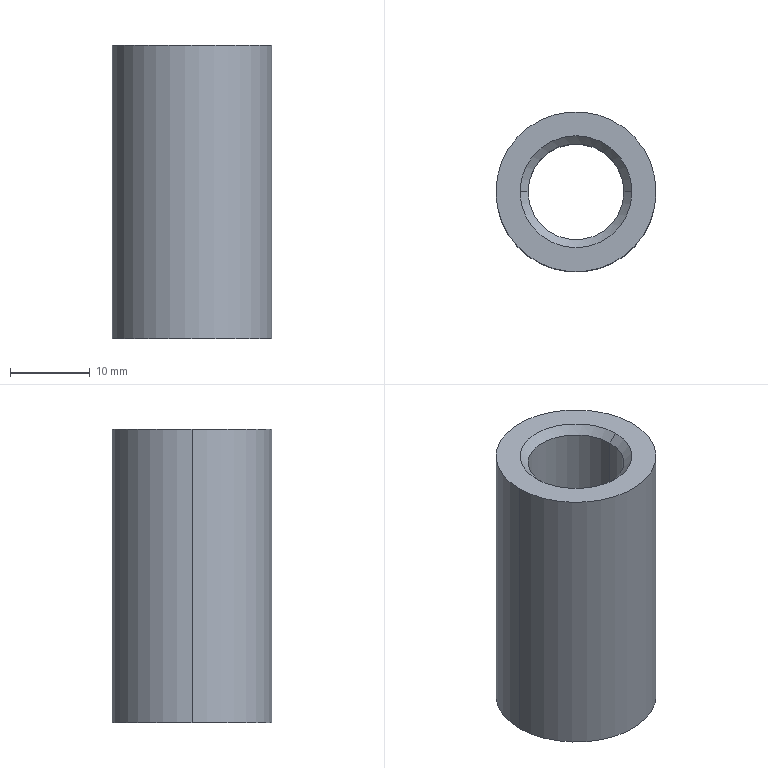Part | STEP file | 塑料轴套内10外20长20 | 1 solid | 10 faces | box 20 x 20 x 36.7 mm | volume 7339 mm3 | cone 4 | cylinder 4 | plane 2 | commonest cylinder face diameters 12 x2 20 x2
STEP:
#1=CARTESIAN_POINT('',(6.,0.,1.));
#2=VERTEX_POINT('',#1);
#3=CARTESIAN_POINT('',(-6.,0.,1.));
#4=VERTEX_POINT('',#3);
#5=CARTESIAN_POINT('',(0.,0.,1.));
#6=DIRECTION('',(0.,0.,-1.));
#7=DIRECTION('',(1.,0.,0.));
#8=AXIS2_PLACEMENT_3D('',#5,#6,#7);
#9=CIRCLE('',#8,6.);
#10=EDGE_CURVE('',#2,#4,#9,.T.);
#11=ORIENTED_EDGE('',*,*,#10,.F.);
#12=CARTESIAN_POINT('',(7.,0.,0.));
#13=VERTEX_POINT('',#12);
#14=CARTESIAN_POINT('',(7.,0.,0.));
#15=DIRECTION('',(0.7071,0.,-0.7071));
#16=VECTOR('',#15,1000.);
#17=LINE('',#14,#16);
#18=EDGE_CURVE('',#2,#13,#17,.T.);
#19=ORIENTED_EDGE('',*,*,#18,.T.);
#20=CARTESIAN_POINT('',(-7.,0.,0.));
#21=VERTEX_POINT('',#20);
#22=CARTESIAN_POINT('',(0.,0.,0.));
#23=DIRECTION('',(0.,0.,1.));
#24=DIRECTION('',(1.,0.,0.));
#25=AXIS2_PLACEMENT_3D('',#22,#23,#24);
#26=CIRCLE('',#25,7.);
#27=EDGE_CURVE('',#21,#13,#26,.T.);
#28=ORIENTED_EDGE('',*,*,#27,.F.);
#29=CARTESIAN_POINT('',(-7.,0.,0.));
#30=DIRECTION('',(-0.7071,0.,-0.7071));
#31=VECTOR('',#30,1000.);
#32=LINE('',#29,#31);
#33=EDGE_CURVE('',#4,#21,#32,.T.);
#34=ORIENTED_EDGE('',*,*,#33,.F.);
#35=EDGE_LOOP('',(#11,#19,#28,#34));
#36=FACE_OUTER_BOUND('',#35,.T.);
#37=CARTESIAN_POINT('',(0.,0.,0.));
#38=DIRECTION('',(0.,0.,-1.));
#39=DIRECTION('',(-1.,0.,0.));
#40=AXIS2_PLACEMENT_3D('',#37,#38,#39);
#41=CONICAL_SURFACE('',#40,7.,0.7854);
#42=ADVANCED_FACE('',(#36),#41,.F.);
#43=CARTESIAN_POINT('',(-6.,0.,35.7));
#44=VERTEX_POINT('',#43);
#45=CARTESIAN_POINT('',(6.,0.,35.7));
#46=VERTEX_POINT('',#45);
#47=CARTESIAN_POINT('',(0.,0.,35.7));
#48=DIRECTION('',(0.,0.,1.));
#49=DIRECTION('',(1.,0.,0.));
#50=AXIS2_PLACEMENT_3D('',#47,#48,#49);
#51=CIRCLE('',#50,6.);
#52=EDGE_CURVE('',#44,#46,#51,.T.);
#53=ORIENTED_EDGE('',*,*,#52,.F.);
#54=CARTESIAN_POINT('',(-7.,0.,36.7));
#55=VERTEX_POINT('',#54);
#56=CARTESIAN_POINT('',(-6.,0.,35.7));
#57=DIRECTION('',(-0.7071,0.,0.7071));
#58=VECTOR('',#57,1000.);
#59=LINE('',#56,#58);
#60=EDGE_CURVE('',#44,#55,#59,.T.);
#61=ORIENTED_EDGE('',*,*,#60,.T.);
#62=CARTESIAN_POINT('',(7.,0.,36.7));
#63=VERTEX_POINT('',#62);
#64=CARTESIAN_POINT('',(0.,0.,36.7));
#65=DIRECTION('',(0.,0.,-1.));
#66=DIRECTION('',(1.,0.,0.));
#67=AXIS2_PLACEMENT_3D('',#64,#65,#66);
#68=CIRCLE('',#67,7.);
#69=EDGE_CURVE('',#63,#55,#68,.T.);
#70=ORIENTED_EDGE('',*,*,#69,.F.);
#71=CARTESIAN_POINT('',(6.,0.,35.7));
#72=DIRECTION('',(0.7071,0.,0.7071));
#73=VECTOR('',#72,1000.);
#74=LINE('',#71,#73);
#75=EDGE_CURVE('',#46,#63,#74,.T.);
#76=ORIENTED_EDGE('',*,*,#75,.F.);
#77=EDGE_LOOP('',(#53,#61,#70,#76));
#78=FACE_OUTER_BOUND('',#77,.T.);
#79=CARTESIAN_POINT('',(0.,0.,35.7));
#80=DIRECTION('',(0.,0.,1.));
#81=DIRECTION('',(1.,0.,0.));
#82=AXIS2_PLACEMENT_3D('',#79,#80,#81);
#83=CONICAL_SURFACE('',#82,6.,0.7854);
#84=ADVANCED_FACE('',(#78),#83,.F.);
#85=ORIENTED_EDGE('',*,*,#52,.T.);
#86=CARTESIAN_POINT('',(6.,0.,36.7));
#87=DIRECTION('',(0.,0.,-1.));
#88=VECTOR('',#87,1000.);
#89=LINE('',#86,#88);
#90=EDGE_CURVE('',#46,#2,#89,.T.);
#91=ORIENTED_EDGE('',*,*,#90,.T.);
#92=ORIENTED_EDGE('',*,*,#10,.T.);
#93=CARTESIAN_POINT('',(-6.,0.,36.7));
#94=DIRECTION('',(0.,0.,-1.));
#95=VECTOR('',#94,1000.);
#96=LINE('',#93,#95);
#97=EDGE_CURVE('',#44,#4,#96,.T.);
#98=ORIENTED_EDGE('',*,*,#97,.F.);
#99=EDGE_LOOP('',(#85,#91,#92,#98));
#100=FACE_OUTER_BOUND('',#99,.T.);
#101=CARTESIAN_POINT('',(0.,0.,36.7));
#102=DIRECTION('',(0.,0.,-1.));
#103=DIRECTION('',(-1.,0.,0.));
#104=AXIS2_PLACEMENT_3D('',#101,#102,#103);
#105=CYLINDRICAL_SURFACE('',#104,6.);
#106=ADVANCED_FACE('',(#100),#105,.F.);
#107=CARTESIAN_POINT('',(10.,0.,36.7));
#108=VERTEX_POINT('',#107);
#109=CARTESIAN_POINT('',(-10.,0.,36.7));
#110=VERTEX_POINT('',#109);
#111=CARTESIAN_POINT('',(0.,0.,36.7));
#112=DIRECTION('',(0.,0.,1.));
#113=DIRECTION('',(1.,0.,0.));
#114=AXIS2_PLACEMENT_3D('',#111,#112,#113);
#115=CIRCLE('',#114,10.);
#116=EDGE_CURVE('',#108,#110,#115,.T.);
#117=ORIENTED_EDGE('',*,*,#116,.F.);
#118=CARTESIAN_POINT('',(10.,0.,0.));
#119=VERTEX_POINT('',#118);
#120=CARTESIAN_POINT('',(10.,0.,36.7));
#121=DIRECTION('',(0.,0.,-1.));
#122=VECTOR('',#121,1000.);
#123=LINE('',#120,#122);
#124=EDGE_CURVE('',#108,#119,#123,.T.);
#125=ORIENTED_EDGE('',*,*,#124,.T.);
#126=CARTESIAN_POINT('',(-10.,0.,0.));
#127=VERTEX_POINT('',#126);
#128=CARTESIAN_POINT('',(0.,0.,0.));
#129=DIRECTION('',(0.,0.,1.));
#130=DIRECTION('',(1.,0.,0.));
#131=AXIS2_PLACEMENT_3D('',#128,#129,#130);
#132=CIRCLE('',#131,10.);
#133=EDGE_CURVE('',#119,#127,#132,.T.);
#134=ORIENTED_EDGE('',*,*,#133,.T.);
#135=CARTESIAN_POINT('',(-10.,0.,36.7));
#136=DIRECTION('',(0.,0.,-1.));
#137=VECTOR('',#136,1000.);
#138=LINE('',#135,#137);
#139=EDGE_CURVE('',#110,#127,#138,.T.);
#140=ORIENTED_EDGE('',*,*,#139,.F.);
#141=EDGE_LOOP('',(#117,#125,#134,#140));
#142=FACE_OUTER_BOUND('',#141,.T.);
#143=CARTESIAN_POINT('',(0.,0.,36.7));
#144=DIRECTION('',(0.,0.,-1.));
#145=DIRECTION('',(-1.,0.,0.));
#146=AXIS2_PLACEMENT_3D('',#143,#144,#145);
#147=CYLINDRICAL_SURFACE('',#146,10.);
#148=ADVANCED_FACE('',(#142),#147,.T.);
#149=ORIENTED_EDGE('',*,*,#69,.T.);
#150=CARTESIAN_POINT('',(0.,0.,36.7));
#151=DIRECTION('',(0.,0.,-1.));
#152=DIRECTION('',(1.,0.,0.));
#153=AXIS2_PLACEMENT_3D('',#150,#151,#152);
#154=CIRCLE('',#153,7.);
#155=EDGE_CURVE('',#55,#63,#154,.T.);
#156=ORIENTED_EDGE('',*,*,#155,.T.);
#157=EDGE_LOOP('',(#149,#156));
#158=FACE_BOUND('',#157,.T.);
#159=CARTESIAN_POINT('',(0.,0.,36.7));
#160=DIRECTION('',(0.,0.,1.));
#161=DIRECTION('',(1.,0.,0.));
#162=AXIS2_PLACEMENT_3D('',#159,#160,#161);
#163=CIRCLE('',#162,10.);
#164=EDGE_CURVE('',#110,#108,#163,.T.);
#165=ORIENTED_EDGE('',*,*,#164,.T.);
#166=ORIENTED_EDGE('',*,*,#116,.T.);
#167=EDGE_LOOP('',(#165,#166));
#168=FACE_OUTER_BOUND('',#167,.T.);
#169=CARTESIAN_POINT('',(0.,0.,36.7));
#170=DIRECTION('',(0.,0.,1.));
#171=DIRECTION('',(1.,0.,0.));
#172=AXIS2_PLACEMENT_3D('',#169,#170,#171);
#173=PLANE('',#172);
#174=ADVANCED_FACE('',(#158,#168),#173,.T.);
#175=ORIENTED_EDGE('',*,*,#27,.T.);
#176=CARTESIAN_POINT('',(0.,0.,0.));
#177=DIRECTION('',(0.,0.,1.));
#178=DIRECTION('',(1.,0.,0.));
#179=AXIS2_PLACEMENT_3D('',#176,#177,#178);
#180=CIRCLE('',#179,7.);
#181=EDGE_CURVE('',#13,#21,#180,.T.);
#182=ORIENTED_EDGE('',*,*,#181,.T.);
#183=EDGE_LOOP('',(#175,#182));
#184=FACE_BOUND('',#183,.T.);
#185=CARTESIAN_POINT('',(0.,0.,0.));
#186=DIRECTION('',(0.,0.,1.));
#187=DIRECTION('',(1.,0.,0.));
#188=AXIS2_PLACEMENT_3D('',#185,#186,#187);
#189=CIRCLE('',#188,10.);
#190=EDGE_CURVE('',#127,#119,#189,.T.);
#191=ORIENTED_EDGE('',*,*,#190,.F.);
#192=ORIENTED_EDGE('',*,*,#133,.F.);
#193=EDGE_LOOP('',(#191,#192));
#194=FACE_OUTER_BOUND('',#193,.T.);
#195=CARTESIAN_POINT('',(0.,0.,0.));
#196=DIRECTION('',(0.,0.,1.));
#197=DIRECTION('',(1.,0.,0.));
#198=AXIS2_PLACEMENT_3D('',#195,#196,#197);
#199=PLANE('',#198);
#200=ADVANCED_FACE('',(#184,#194),#199,.F.);
#201=ORIENTED_EDGE('',*,*,#124,.F.);
#202=ORIENTED_EDGE('',*,*,#164,.F.);
#203=ORIENTED_EDGE('',*,*,#139,.T.);
#204=ORIENTED_EDGE('',*,*,#190,.T.);
#205=EDGE_LOOP('',(#201,#202,#203,#204));
#206=FACE_OUTER_BOUND('',#205,.T.);
#207=CARTESIAN_POINT('',(0.,0.,36.7));
#208=DIRECTION('',(0.,0.,-1.));
#209=DIRECTION('',(-1.,0.,0.));
#210=AXIS2_PLACEMENT_3D('',#207,#208,#209);
#211=CYLINDRICAL_SURFACE('',#210,10.);
#212=ADVANCED_FACE('',(#206),#211,.T.);
#213=ORIENTED_EDGE('',*,*,#90,.F.);
#214=CARTESIAN_POINT('',(0.,0.,35.7));
#215=DIRECTION('',(0.,0.,1.));
#216=DIRECTION('',(1.,0.,0.));
#217=AXIS2_PLACEMENT_3D('',#214,#215,#216);
#218=CIRCLE('',#217,6.);
#219=EDGE_CURVE('',#46,#44,#218,.T.);
#220=ORIENTED_EDGE('',*,*,#219,.T.);
#221=ORIENTED_EDGE('',*,*,#97,.T.);
#222=CARTESIAN_POINT('',(0.,0.,1.));
#223=DIRECTION('',(0.,0.,-1.));
#224=DIRECTION('',(1.,0.,0.));
#225=AXIS2_PLACEMENT_3D('',#222,#223,#224);
#226=CIRCLE('',#225,6.);
#227=EDGE_CURVE('',#4,#2,#226,.T.);
#228=ORIENTED_EDGE('',*,*,#227,.T.);
#229=EDGE_LOOP('',(#213,#220,#221,#228));
#230=FACE_OUTER_BOUND('',#229,.T.);
#231=CARTESIAN_POINT('',(0.,0.,36.7));
#232=DIRECTION('',(0.,0.,-1.));
#233=DIRECTION('',(-1.,0.,0.));
#234=AXIS2_PLACEMENT_3D('',#231,#232,#233);
#235=CYLINDRICAL_SURFACE('',#234,6.);
#236=ADVANCED_FACE('',(#230),#235,.F.);
#237=ORIENTED_EDGE('',*,*,#60,.F.);
#238=ORIENTED_EDGE('',*,*,#219,.F.);
#239=ORIENTED_EDGE('',*,*,#75,.T.);
#240=ORIENTED_EDGE('',*,*,#155,.F.);
#241=EDGE_LOOP('',(#237,#238,#239,#240));
#242=FACE_OUTER_BOUND('',#241,.T.);
#243=CARTESIAN_POINT('',(0.,0.,35.7));
#244=DIRECTION('',(0.,0.,1.));
#245=DIRECTION('',(1.,0.,0.));
#246=AXIS2_PLACEMENT_3D('',#243,#244,#245);
#247=CONICAL_SURFACE('',#246,6.,0.7854);
#248=ADVANCED_FACE('',(#242),#247,.F.);
#249=ORIENTED_EDGE('',*,*,#18,.F.);
#250=ORIENTED_EDGE('',*,*,#227,.F.);
#251=ORIENTED_EDGE('',*,*,#33,.T.);
#252=ORIENTED_EDGE('',*,*,#181,.F.);
#253=EDGE_LOOP('',(#249,#250,#251,#252));
#254=FACE_OUTER_BOUND('',#253,.T.);
#255=CARTESIAN_POINT('',(0.,0.,0.));
#256=DIRECTION('',(0.,0.,-1.));
#257=DIRECTION('',(-1.,0.,0.));
#258=AXIS2_PLACEMENT_3D('',#255,#256,#257);
#259=CONICAL_SURFACE('',#258,7.,0.7854);
#260=ADVANCED_FACE('',(#254),#259,.F.);
#261=CLOSED_SHELL('',(#42,#84,#106,#148,#174,#200,#212,#236,#248,#260));
#262=MANIFOLD_SOLID_BREP('',#261);
#263=CARTESIAN_POINT('',(0.,0.,0.));
#264=DIRECTION('',(0.,0.,1.));
#265=DIRECTION('',(1.,0.,0.));
#266=AXIS2_PLACEMENT_3D('',#263,#264,#265);
#267=(LENGTH_UNIT()NAMED_UNIT(*)SI_UNIT(.MILLI.,.METRE.));
#268=UNCERTAINTY_MEASURE_WITH_UNIT(LENGTH_MEASURE(0.00001),#267,'','');
#269=(NAMED_UNIT(*)PLANE_ANGLE_UNIT()SI_UNIT($,.RADIAN.));
#270=(NAMED_UNIT(*)SI_UNIT($,.STERADIAN.)SOLID_ANGLE_UNIT());
#271=(GEOMETRIC_REPRESENTATION_CONTEXT(3)GLOBAL_UNCERTAINTY_ASSIGNED_CONTEXT((#268))GLOBAL_UNIT_ASSIGNED_CONTEXT((#267,#269,#270))REPRESENTATION_CONTEXT('',''));
#272=ADVANCED_BREP_SHAPE_REPRESENTATION('',(#262,#266),#271);